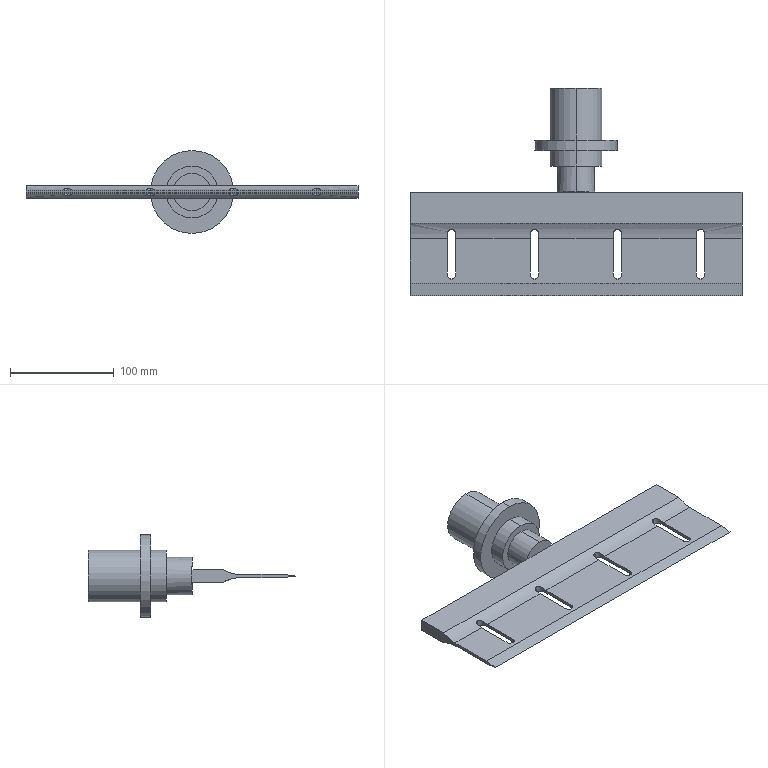Part | STEP file | 1 solid | 46 faces | box 320 x 200 x 80 mm | volume 390081 mm3 | plane 24 | cylinder 20 | spline 2 | commonest cylinder face diameters 8 x12 50 x4 36 x2 80 x2